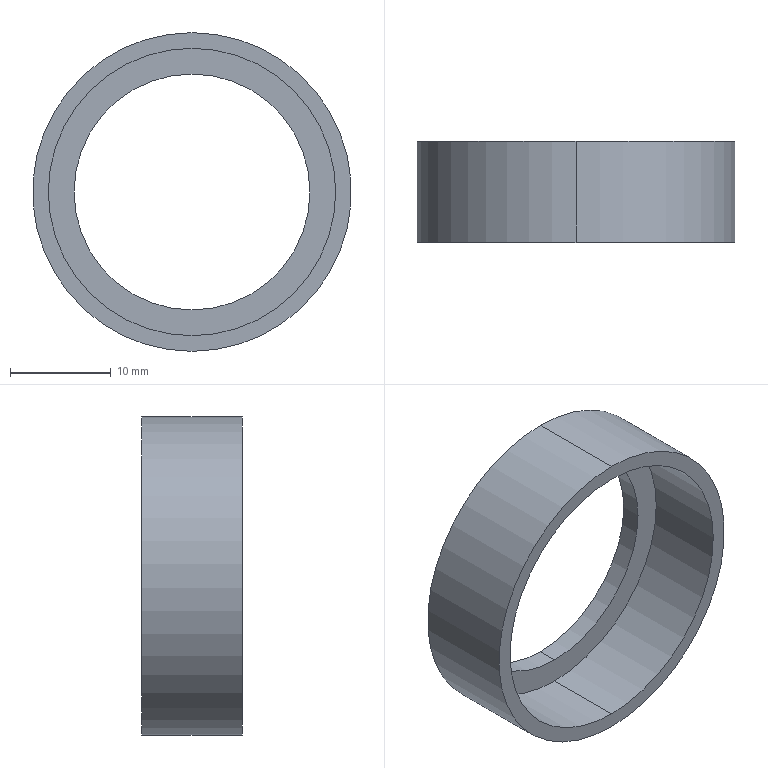Part | STEP file | P2858E27_RING_DICHT | 1 solid | 9 faces | box 31.6 x 10 x 31.6 mm | volume 1879 mm3 | cylinder 6 | plane 3 | commonest cylinder face diameters 23.4 x2 28.5 x2 31.6 x2
STEP:
#1=CARTESIAN_POINT('',(0.,0.,0.));
#2=DIRECTION('',(0.,0.,1.));
#3=DIRECTION('',(1.,0.,0.));
#4=AXIS2_PLACEMENT_3D('',#1,#2,#3);
#5=CARTESIAN_POINT('',(0.,28.,-15.8));
#6=VERTEX_POINT('',#5);
#7=CARTESIAN_POINT('',(0.,28.,15.8));
#8=VERTEX_POINT('',#7);
#9=CARTESIAN_POINT('',(0.,28.,0.));
#10=DIRECTION('',(0.,-1.,0.));
#11=DIRECTION('',(0.,0.,-1.));
#12=AXIS2_PLACEMENT_3D('',#9,#10,#11);
#13=CIRCLE('',#12,15.8);
#14=CARTESIAN_POINT('',(0.,23.,0.));
#15=DIRECTION('',(0.,-1.,0.));
#16=DIRECTION('',(0.,0.,-1.));
#17=AXIS2_PLACEMENT_3D('',#14,#15,#16);
#18=CYLINDRICAL_SURFACE('',#17,15.8);
#19=CARTESIAN_POINT('',(0.,-5.));
#20=DIRECTION('',(1.,0.));
#21=VECTOR('',#20,1.);
#22=LINE('',#19,#21);
#23=(GEOMETRIC_REPRESENTATION_CONTEXT(2)PARAMETRIC_REPRESENTATION_CONTEXT()REPRESENTATION_CONTEXT('',''));
#24=DEFINITIONAL_REPRESENTATION('',(#22),#23);
#25=PCURVE('',#18,#24);
#26=CARTESIAN_POINT('',(-13.75,28.,0.));
#27=DIRECTION('',(0.,-1.,0.));
#28=DIRECTION('',(0.,0.,-1.));
#29=AXIS2_PLACEMENT_3D('',#26,#27,#28);
#30=PLANE('',#29);
#31=CARTESIAN_POINT('',(0.,13.75));
#32=DIRECTION('',(1.,0.));
#33=AXIS2_PLACEMENT_2D('',#31,#32);
#34=CIRCLE('',#33,15.8);
#35=(GEOMETRIC_REPRESENTATION_CONTEXT(2)PARAMETRIC_REPRESENTATION_CONTEXT()REPRESENTATION_CONTEXT('',''));
#36=DEFINITIONAL_REPRESENTATION('',(#34),#35);
#37=PCURVE('',#30,#36);
#38=SURFACE_CURVE('',#13,(#25,#37),.PCURVE_S1.);
#39=EDGE_CURVE('',#6,#8,#38,.T.);
#40=ORIENTED_EDGE('',*,*,#39,.T.);
#41=CARTESIAN_POINT('',(0.,18.,15.8));
#42=VERTEX_POINT('',#41);
#43=CARTESIAN_POINT('',(0.,23.,15.8));
#44=DIRECTION('',(0.,-1.,0.));
#45=VECTOR('',#44,1.);
#46=LINE('',#43,#45);
#47=CARTESIAN_POINT('',(3.142,0.));
#48=DIRECTION('',(0.,1.));
#49=VECTOR('',#48,1.);
#50=LINE('',#47,#49);
#51=(GEOMETRIC_REPRESENTATION_CONTEXT(2)PARAMETRIC_REPRESENTATION_CONTEXT()REPRESENTATION_CONTEXT('',''));
#52=DEFINITIONAL_REPRESENTATION('',(#50),#51);
#53=PCURVE('',#18,#52);
#54=CARTESIAN_POINT('',(0.,23.,0.));
#55=DIRECTION('',(0.,-1.,0.));
#56=DIRECTION('',(0.,0.,-1.));
#57=AXIS2_PLACEMENT_3D('',#54,#55,#56);
#58=CYLINDRICAL_SURFACE('',#57,15.8);
#59=CARTESIAN_POINT('',(3.142,0.));
#60=DIRECTION('',(0.,1.));
#61=VECTOR('',#60,1.);
#62=LINE('',#59,#61);
#63=(GEOMETRIC_REPRESENTATION_CONTEXT(2)PARAMETRIC_REPRESENTATION_CONTEXT()REPRESENTATION_CONTEXT('',''));
#64=DEFINITIONAL_REPRESENTATION('',(#62),#63);
#65=PCURVE('',#58,#64);
#66=SURFACE_CURVE('',#46,(#53,#65),.PCURVE_S1.);
#67=EDGE_CURVE('',#8,#42,#66,.T.);
#68=ORIENTED_EDGE('',*,*,#67,.T.);
#69=CARTESIAN_POINT('',(0.,18.,-15.8));
#70=VERTEX_POINT('',#69);
#71=CARTESIAN_POINT('',(0.,18.,0.));
#72=DIRECTION('',(0.,1.,0.));
#73=DIRECTION('',(0.,0.,-1.));
#74=AXIS2_PLACEMENT_3D('',#71,#72,#73);
#75=CIRCLE('',#74,15.8);
#76=CARTESIAN_POINT('',(6.283,5.));
#77=DIRECTION('',(-1.,0.));
#78=VECTOR('',#77,1.);
#79=LINE('',#76,#78);
#80=(GEOMETRIC_REPRESENTATION_CONTEXT(2)PARAMETRIC_REPRESENTATION_CONTEXT()REPRESENTATION_CONTEXT('',''));
#81=DEFINITIONAL_REPRESENTATION('',(#79),#80);
#82=PCURVE('',#18,#81);
#83=CARTESIAN_POINT('',(-15.025,18.,0.));
#84=DIRECTION('',(0.,-1.,0.));
#85=DIRECTION('',(0.,0.,-1.));
#86=AXIS2_PLACEMENT_3D('',#83,#84,#85);
#87=PLANE('',#86);
#88=CARTESIAN_POINT('',(15.8,15.025));
#89=CARTESIAN_POINT('',(15.8,-12.341));
#90=CARTESIAN_POINT('',(-7.9,1.342));
#91=CARTESIAN_POINT('',(-31.6,15.025));
#92=CARTESIAN_POINT('',(-7.9,28.708));
#93=CARTESIAN_POINT('',(15.8,42.391));
#94=CARTESIAN_POINT('',(15.8,15.025));
#95=(BOUNDED_CURVE()B_SPLINE_CURVE(2,(#88,#89,#90,#91,#92,#93,#94),.UNSPECIFIED.,.T.,.F.)B_SPLINE_CURVE_WITH_KNOTS((1,2,2,2,2,1),(-2.094,0.,2.094,4.189,6.283,8.378),.UNSPECIFIED.)CURVE()GEOMETRIC_REPRESENTATION_ITEM()RATIONAL_B_SPLINE_CURVE((1.,0.5,1.,0.5,1.,0.5,1.))REPRESENTATION_ITEM(''));
#96=(GEOMETRIC_REPRESENTATION_CONTEXT(2)PARAMETRIC_REPRESENTATION_CONTEXT()REPRESENTATION_CONTEXT('',''));
#97=DEFINITIONAL_REPRESENTATION('',(#95),#96);
#98=PCURVE('',#87,#97);
#99=SURFACE_CURVE('',#75,(#82,#98),.PCURVE_S1.);
#100=EDGE_CURVE('',#42,#70,#99,.T.);
#101=ORIENTED_EDGE('',*,*,#100,.T.);
#102=CARTESIAN_POINT('',(0.,23.,-15.8));
#103=DIRECTION('',(0.,-1.,0.));
#104=VECTOR('',#103,1.);
#105=LINE('',#102,#104);
#106=CARTESIAN_POINT('',(0.,0.));
#107=DIRECTION('',(0.,1.));
#108=VECTOR('',#107,1.);
#109=LINE('',#106,#108);
#110=(GEOMETRIC_REPRESENTATION_CONTEXT(2)PARAMETRIC_REPRESENTATION_CONTEXT()REPRESENTATION_CONTEXT('',''));
#111=DEFINITIONAL_REPRESENTATION('',(#109),#110);
#112=PCURVE('',#18,#111);
#113=CARTESIAN_POINT('',(6.283,0.));
#114=DIRECTION('',(0.,1.));
#115=VECTOR('',#114,1.);
#116=LINE('',#113,#115);
#117=(GEOMETRIC_REPRESENTATION_CONTEXT(2)PARAMETRIC_REPRESENTATION_CONTEXT()REPRESENTATION_CONTEXT('',''));
#118=DEFINITIONAL_REPRESENTATION('',(#116),#117);
#119=PCURVE('',#58,#118);
#120=SURFACE_CURVE('',#105,(#112,#119),.PCURVE_S1.);
#121=EDGE_CURVE('',#6,#70,#120,.T.);
#122=ORIENTED_EDGE('',*,*,#121,.F.);
#123=EDGE_LOOP('',(#40,#68,#101,#122));
#124=FACE_BOUND('',#123,.T.);
#125=ADVANCED_FACE('',(#124),#18,.T.);
#126=CARTESIAN_POINT('',(0.,28.,-11.7));
#127=VERTEX_POINT('',#126);
#128=CARTESIAN_POINT('',(0.,26.,-11.7));
#129=VERTEX_POINT('',#128);
#130=CARTESIAN_POINT('',(0.,27.,-11.7));
#131=DIRECTION('',(0.,-1.,0.));
#132=VECTOR('',#131,1.);
#133=LINE('',#130,#132);
#134=CARTESIAN_POINT('',(0.,27.,0.));
#135=DIRECTION('',(0.,-1.,0.));
#136=DIRECTION('',(0.,0.,-1.));
#137=AXIS2_PLACEMENT_3D('',#134,#135,#136);
#138=CYLINDRICAL_SURFACE('',#137,11.7);
#139=CARTESIAN_POINT('',(6.283,0.));
#140=DIRECTION('',(0.,1.));
#141=VECTOR('',#140,1.);
#142=LINE('',#139,#141);
#143=(GEOMETRIC_REPRESENTATION_CONTEXT(2)PARAMETRIC_REPRESENTATION_CONTEXT()REPRESENTATION_CONTEXT('',''));
#144=DEFINITIONAL_REPRESENTATION('',(#142),#143);
#145=PCURVE('',#138,#144);
#146=CARTESIAN_POINT('',(0.,27.,0.));
#147=DIRECTION('',(0.,-1.,0.));
#148=DIRECTION('',(0.,0.,-1.));
#149=AXIS2_PLACEMENT_3D('',#146,#147,#148);
#150=CYLINDRICAL_SURFACE('',#149,11.7);
#151=CARTESIAN_POINT('',(0.,0.));
#152=DIRECTION('',(0.,1.));
#153=VECTOR('',#152,1.);
#154=LINE('',#151,#153);
#155=(GEOMETRIC_REPRESENTATION_CONTEXT(2)PARAMETRIC_REPRESENTATION_CONTEXT()REPRESENTATION_CONTEXT('',''));
#156=DEFINITIONAL_REPRESENTATION('',(#154),#155);
#157=PCURVE('',#150,#156);
#158=SURFACE_CURVE('',#133,(#145,#157),.PCURVE_S1.);
#159=EDGE_CURVE('',#127,#129,#158,.T.);
#160=ORIENTED_EDGE('',*,*,#159,.T.);
#161=CARTESIAN_POINT('',(0.,26.,11.7));
#162=VERTEX_POINT('',#161);
#163=CARTESIAN_POINT('',(0.,26.,0.));
#164=DIRECTION('',(0.,1.,0.));
#165=DIRECTION('',(0.,0.,-1.));
#166=AXIS2_PLACEMENT_3D('',#163,#164,#165);
#167=CIRCLE('',#166,11.7);
#168=CARTESIAN_POINT('',(6.283,1.));
#169=DIRECTION('',(-1.,0.));
#170=VECTOR('',#169,1.);
#171=LINE('',#168,#170);
#172=(GEOMETRIC_REPRESENTATION_CONTEXT(2)PARAMETRIC_REPRESENTATION_CONTEXT()REPRESENTATION_CONTEXT('',''));
#173=DEFINITIONAL_REPRESENTATION('',(#171),#172);
#174=PCURVE('',#138,#173);
#175=CARTESIAN_POINT('',(-12.975,26.,0.));
#176=DIRECTION('',(0.,-1.,0.));
#177=DIRECTION('',(0.,0.,-1.));
#178=AXIS2_PLACEMENT_3D('',#175,#176,#177);
#179=PLANE('',#178);
#180=CARTESIAN_POINT('',(11.7,12.975));
#181=CARTESIAN_POINT('',(11.7,-7.29));
#182=CARTESIAN_POINT('',(-5.85,2.843));
#183=CARTESIAN_POINT('',(-23.4,12.975));
#184=CARTESIAN_POINT('',(-5.85,23.107));
#185=CARTESIAN_POINT('',(11.7,33.24));
#186=CARTESIAN_POINT('',(11.7,12.975));
#187=(BOUNDED_CURVE()B_SPLINE_CURVE(2,(#180,#181,#182,#183,#184,#185,#186),.UNSPECIFIED.,.T.,.F.)B_SPLINE_CURVE_WITH_KNOTS((1,2,2,2,2,1),(-2.094,0.,2.094,4.189,6.283,8.378),.UNSPECIFIED.)CURVE()GEOMETRIC_REPRESENTATION_ITEM()RATIONAL_B_SPLINE_CURVE((1.,0.5,1.,0.5,1.,0.5,1.))REPRESENTATION_ITEM(''));
#188=(GEOMETRIC_REPRESENTATION_CONTEXT(2)PARAMETRIC_REPRESENTATION_CONTEXT()REPRESENTATION_CONTEXT('',''));
#189=DEFINITIONAL_REPRESENTATION('',(#187),#188);
#190=PCURVE('',#179,#189);
#191=SURFACE_CURVE('',#167,(#174,#190),.PCURVE_S1.);
#192=EDGE_CURVE('',#129,#162,#191,.T.);
#193=ORIENTED_EDGE('',*,*,#192,.T.);
#194=CARTESIAN_POINT('',(0.,28.,11.7));
#195=VERTEX_POINT('',#194);
#196=CARTESIAN_POINT('',(0.,27.,11.7));
#197=DIRECTION('',(0.,-1.,0.));
#198=VECTOR('',#197,1.);
#199=LINE('',#196,#198);
#200=CARTESIAN_POINT('',(3.142,0.));
#201=DIRECTION('',(0.,1.));
#202=VECTOR('',#201,1.);
#203=LINE('',#200,#202);
#204=(GEOMETRIC_REPRESENTATION_CONTEXT(2)PARAMETRIC_REPRESENTATION_CONTEXT()REPRESENTATION_CONTEXT('',''));
#205=DEFINITIONAL_REPRESENTATION('',(#203),#204);
#206=PCURVE('',#138,#205);
#207=CARTESIAN_POINT('',(3.142,0.));
#208=DIRECTION('',(0.,1.));
#209=VECTOR('',#208,1.);
#210=LINE('',#207,#209);
#211=(GEOMETRIC_REPRESENTATION_CONTEXT(2)PARAMETRIC_REPRESENTATION_CONTEXT()REPRESENTATION_CONTEXT('',''));
#212=DEFINITIONAL_REPRESENTATION('',(#210),#211);
#213=PCURVE('',#150,#212);
#214=SURFACE_CURVE('',#199,(#206,#213),.PCURVE_S1.);
#215=EDGE_CURVE('',#195,#162,#214,.T.);
#216=ORIENTED_EDGE('',*,*,#215,.F.);
#217=CARTESIAN_POINT('',(0.,28.,0.));
#218=DIRECTION('',(0.,1.,0.));
#219=DIRECTION('',(0.,0.,-1.));
#220=AXIS2_PLACEMENT_3D('',#217,#218,#219);
#221=CIRCLE('',#220,11.7);
#222=CARTESIAN_POINT('',(6.283,-1.));
#223=DIRECTION('',(-1.,0.));
#224=VECTOR('',#223,1.);
#225=LINE('',#222,#224);
#226=(GEOMETRIC_REPRESENTATION_CONTEXT(2)PARAMETRIC_REPRESENTATION_CONTEXT()REPRESENTATION_CONTEXT('',''));
#227=DEFINITIONAL_REPRESENTATION('',(#225),#226);
#228=PCURVE('',#138,#227);
#229=CARTESIAN_POINT('',(11.7,13.75));
#230=CARTESIAN_POINT('',(11.7,-6.515));
#231=CARTESIAN_POINT('',(-5.85,3.618));
#232=CARTESIAN_POINT('',(-23.4,13.75));
#233=CARTESIAN_POINT('',(-5.85,23.882));
#234=CARTESIAN_POINT('',(11.7,34.015));
#235=CARTESIAN_POINT('',(11.7,13.75));
#236=(BOUNDED_CURVE()B_SPLINE_CURVE(2,(#229,#230,#231,#232,#233,#234,#235),.UNSPECIFIED.,.T.,.F.)B_SPLINE_CURVE_WITH_KNOTS((1,2,2,2,2,1),(-2.094,0.,2.094,4.189,6.283,8.378),.UNSPECIFIED.)CURVE()GEOMETRIC_REPRESENTATION_ITEM()RATIONAL_B_SPLINE_CURVE((1.,0.5,1.,0.5,1.,0.5,1.))REPRESENTATION_ITEM(''));
#237=(GEOMETRIC_REPRESENTATION_CONTEXT(2)PARAMETRIC_REPRESENTATION_CONTEXT()REPRESENTATION_CONTEXT('',''));
#238=DEFINITIONAL_REPRESENTATION('',(#236),#237);
#239=PCURVE('',#30,#238);
#240=SURFACE_CURVE('',#221,(#228,#239),.PCURVE_S1.);
#241=EDGE_CURVE('',#127,#195,#240,.T.);
#242=ORIENTED_EDGE('',*,*,#241,.F.);
#243=EDGE_LOOP('',(#160,#193,#216,#242));
#244=FACE_BOUND('',#243,.F.);
#245=ADVANCED_FACE('',(#244),#138,.F.);
#246=CARTESIAN_POINT('',(0.,26.,-14.25));
#247=VERTEX_POINT('',#246);
#248=CARTESIAN_POINT('',(0.,18.,-14.25));
#249=VERTEX_POINT('',#248);
#250=CARTESIAN_POINT('',(0.,22.,-14.25));
#251=DIRECTION('',(0.,-1.,0.));
#252=VECTOR('',#251,1.);
#253=LINE('',#250,#252);
#254=CARTESIAN_POINT('',(0.,22.,0.));
#255=DIRECTION('',(0.,-1.,0.));
#256=DIRECTION('',(0.,0.,-1.));
#257=AXIS2_PLACEMENT_3D('',#254,#255,#256);
#258=CYLINDRICAL_SURFACE('',#257,14.25);
#259=CARTESIAN_POINT('',(6.283,0.));
#260=DIRECTION('',(0.,1.));
#261=VECTOR('',#260,1.);
#262=LINE('',#259,#261);
#263=(GEOMETRIC_REPRESENTATION_CONTEXT(2)PARAMETRIC_REPRESENTATION_CONTEXT()REPRESENTATION_CONTEXT('',''));
#264=DEFINITIONAL_REPRESENTATION('',(#262),#263);
#265=PCURVE('',#258,#264);
#266=CARTESIAN_POINT('',(0.,22.,0.));
#267=DIRECTION('',(0.,-1.,0.));
#268=DIRECTION('',(0.,0.,-1.));
#269=AXIS2_PLACEMENT_3D('',#266,#267,#268);
#270=CYLINDRICAL_SURFACE('',#269,14.25);
#271=CARTESIAN_POINT('',(0.,0.));
#272=DIRECTION('',(0.,1.));
#273=VECTOR('',#272,1.);
#274=LINE('',#271,#273);
#275=(GEOMETRIC_REPRESENTATION_CONTEXT(2)PARAMETRIC_REPRESENTATION_CONTEXT()REPRESENTATION_CONTEXT('',''));
#276=DEFINITIONAL_REPRESENTATION('',(#274),#275);
#277=PCURVE('',#270,#276);
#278=SURFACE_CURVE('',#253,(#265,#277),.PCURVE_S1.);
#279=EDGE_CURVE('',#247,#249,#278,.T.);
#280=ORIENTED_EDGE('',*,*,#279,.T.);
#281=CARTESIAN_POINT('',(0.,18.,14.25));
#282=VERTEX_POINT('',#281);
#283=CARTESIAN_POINT('',(0.,18.,0.));
#284=DIRECTION('',(0.,1.,0.));
#285=DIRECTION('',(0.,0.,-1.));
#286=AXIS2_PLACEMENT_3D('',#283,#284,#285);
#287=CIRCLE('',#286,14.25);
#288=CARTESIAN_POINT('',(6.283,4.));
#289=DIRECTION('',(-1.,0.));
#290=VECTOR('',#289,1.);
#291=LINE('',#288,#290);
#292=(GEOMETRIC_REPRESENTATION_CONTEXT(2)PARAMETRIC_REPRESENTATION_CONTEXT()REPRESENTATION_CONTEXT('',''));
#293=DEFINITIONAL_REPRESENTATION('',(#291),#292);
#294=PCURVE('',#258,#293);
#295=CARTESIAN_POINT('',(14.25,15.025));
#296=CARTESIAN_POINT('',(14.25,-9.657));
#297=CARTESIAN_POINT('',(-7.125,2.684));
#298=CARTESIAN_POINT('',(-28.5,15.025));
#299=CARTESIAN_POINT('',(-7.125,27.366));
#300=CARTESIAN_POINT('',(14.25,39.707));
#301=CARTESIAN_POINT('',(14.25,15.025));
#302=(BOUNDED_CURVE()B_SPLINE_CURVE(2,(#295,#296,#297,#298,#299,#300,#301),.UNSPECIFIED.,.T.,.F.)B_SPLINE_CURVE_WITH_KNOTS((1,2,2,2,2,1),(-2.094,0.,2.094,4.189,6.283,8.378),.UNSPECIFIED.)CURVE()GEOMETRIC_REPRESENTATION_ITEM()RATIONAL_B_SPLINE_CURVE((1.,0.5,1.,0.5,1.,0.5,1.))REPRESENTATION_ITEM(''));
#303=(GEOMETRIC_REPRESENTATION_CONTEXT(2)PARAMETRIC_REPRESENTATION_CONTEXT()REPRESENTATION_CONTEXT('',''));
#304=DEFINITIONAL_REPRESENTATION('',(#302),#303);
#305=PCURVE('',#87,#304);
#306=SURFACE_CURVE('',#287,(#294,#305),.PCURVE_S1.);
#307=EDGE_CURVE('',#249,#282,#306,.T.);
#308=ORIENTED_EDGE('',*,*,#307,.T.);
#309=CARTESIAN_POINT('',(0.,26.,14.25));
#310=VERTEX_POINT('',#309);
#311=CARTESIAN_POINT('',(0.,22.,14.25));
#312=DIRECTION('',(0.,-1.,0.));
#313=VECTOR('',#312,1.);
#314=LINE('',#311,#313);
#315=CARTESIAN_POINT('',(3.142,0.));
#316=DIRECTION('',(0.,1.));
#317=VECTOR('',#316,1.);
#318=LINE('',#315,#317);
#319=(GEOMETRIC_REPRESENTATION_CONTEXT(2)PARAMETRIC_REPRESENTATION_CONTEXT()REPRESENTATION_CONTEXT('',''));
#320=DEFINITIONAL_REPRESENTATION('',(#318),#319);
#321=PCURVE('',#258,#320);
#322=CARTESIAN_POINT('',(3.142,0.));
#323=DIRECTION('',(0.,1.));
#324=VECTOR('',#323,1.);
#325=LINE('',#322,#324);
#326=(GEOMETRIC_REPRESENTATION_CONTEXT(2)PARAMETRIC_REPRESENTATION_CONTEXT()REPRESENTATION_CONTEXT('',''));
#327=DEFINITIONAL_REPRESENTATION('',(#325),#326);
#328=PCURVE('',#270,#327);
#329=SURFACE_CURVE('',#314,(#321,#328),.PCURVE_S1.);
#330=EDGE_CURVE('',#310,#282,#329,.T.);
#331=ORIENTED_EDGE('',*,*,#330,.F.);
#332=CARTESIAN_POINT('',(0.,26.,0.));
#333=DIRECTION('',(0.,-1.,0.));
#334=DIRECTION('',(0.,0.,-1.));
#335=AXIS2_PLACEMENT_3D('',#332,#333,#334);
#336=CIRCLE('',#335,14.25);
#337=CARTESIAN_POINT('',(0.,-4.));
#338=DIRECTION('',(1.,0.));
#339=VECTOR('',#338,1.);
#340=LINE('',#337,#339);
#341=(GEOMETRIC_REPRESENTATION_CONTEXT(2)PARAMETRIC_REPRESENTATION_CONTEXT()REPRESENTATION_CONTEXT('',''));
#342=DEFINITIONAL_REPRESENTATION('',(#340),#341);
#343=PCURVE('',#258,#342);
#344=CARTESIAN_POINT('',(0.,12.975));
#345=DIRECTION('',(1.,0.));
#346=AXIS2_PLACEMENT_2D('',#344,#345);
#347=CIRCLE('',#346,14.25);
#348=(GEOMETRIC_REPRESENTATION_CONTEXT(2)PARAMETRIC_REPRESENTATION_CONTEXT()REPRESENTATION_CONTEXT('',''));
#349=DEFINITIONAL_REPRESENTATION('',(#347),#348);
#350=PCURVE('',#179,#349);
#351=SURFACE_CURVE('',#336,(#343,#350),.PCURVE_S1.);
#352=EDGE_CURVE('',#310,#247,#351,.T.);
#353=ORIENTED_EDGE('',*,*,#352,.T.);
#354=EDGE_LOOP('',(#280,#308,#331,#353));
#355=FACE_BOUND('',#354,.F.);
#356=ADVANCED_FACE('',(#355),#258,.F.);
#357=ORIENTED_EDGE('',*,*,#192,.T.);
#358=CARTESIAN_POINT('',(0.,26.,0.));
#359=DIRECTION('',(0.,1.,0.));
#360=DIRECTION('',(0.,0.,-1.));
#361=AXIS2_PLACEMENT_3D('',#358,#359,#360);
#362=CIRCLE('',#361,11.7);
#363=CARTESIAN_POINT('',(11.7,12.975));
#364=CARTESIAN_POINT('',(11.7,-7.29));
#365=CARTESIAN_POINT('',(-5.85,2.843));
#366=CARTESIAN_POINT('',(-23.4,12.975));
#367=CARTESIAN_POINT('',(-5.85,23.107));
#368=CARTESIAN_POINT('',(11.7,33.24));
#369=CARTESIAN_POINT('',(11.7,12.975));
#370=(BOUNDED_CURVE()B_SPLINE_CURVE(2,(#363,#364,#365,#366,#367,#368,#369),.UNSPECIFIED.,.T.,.F.)B_SPLINE_CURVE_WITH_KNOTS((1,2,2,2,2,1),(-2.094,0.,2.094,4.189,6.283,8.378),.UNSPECIFIED.)CURVE()GEOMETRIC_REPRESENTATION_ITEM()RATIONAL_B_SPLINE_CURVE((1.,0.5,1.,0.5,1.,0.5,1.))REPRESENTATION_ITEM(''));
#371=(GEOMETRIC_REPRESENTATION_CONTEXT(2)PARAMETRIC_REPRESENTATION_CONTEXT()REPRESENTATION_CONTEXT('',''));
#372=DEFINITIONAL_REPRESENTATION('',(#370),#371);
#373=PCURVE('',#179,#372);
#374=CARTESIAN_POINT('',(6.283,1.));
#375=DIRECTION('',(-1.,0.));
#376=VECTOR('',#375,1.);
#377=LINE('',#374,#376);
#378=(GEOMETRIC_REPRESENTATION_CONTEXT(2)PARAMETRIC_REPRESENTATION_CONTEXT()REPRESENTATION_CONTEXT('',''));
#379=DEFINITIONAL_REPRESENTATION('',(#377),#378);
#380=PCURVE('',#150,#379);
#381=SURFACE_CURVE('',#362,(#373,#380),.PCURVE_S1.);
#382=EDGE_CURVE('',#162,#129,#381,.T.);
#383=ORIENTED_EDGE('',*,*,#382,.T.);
#384=EDGE_LOOP('',(#357,#383));
#385=FACE_BOUND('',#384,.T.);
#386=CARTESIAN_POINT('',(0.,26.,0.));
#387=DIRECTION('',(0.,-1.,0.));
#388=DIRECTION('',(0.,0.,-1.));
#389=AXIS2_PLACEMENT_3D('',#386,#387,#388);
#390=CIRCLE('',#389,14.25);
#391=CARTESIAN_POINT('',(0.,12.975));
#392=DIRECTION('',(1.,0.));
#393=AXIS2_PLACEMENT_2D('',#391,#392);
#394=CIRCLE('',#393,14.25);
#395=(GEOMETRIC_REPRESENTATION_CONTEXT(2)PARAMETRIC_REPRESENTATION_CONTEXT()REPRESENTATION_CONTEXT('',''));
#396=DEFINITIONAL_REPRESENTATION('',(#394),#395);
#397=PCURVE('',#179,#396);
#398=CARTESIAN_POINT('',(0.,-4.));
#399=DIRECTION('',(1.,0.));
#400=VECTOR('',#399,1.);
#401=LINE('',#398,#400);
#402=(GEOMETRIC_REPRESENTATION_CONTEXT(2)PARAMETRIC_REPRESENTATION_CONTEXT()REPRESENTATION_CONTEXT('',''));
#403=DEFINITIONAL_REPRESENTATION('',(#401),#402);
#404=PCURVE('',#270,#403);
#405=SURFACE_CURVE('',#390,(#397,#404),.PCURVE_S1.);
#406=EDGE_CURVE('',#247,#310,#405,.T.);
#407=ORIENTED_EDGE('',*,*,#406,.T.);
#408=ORIENTED_EDGE('',*,*,#352,.T.);
#409=EDGE_LOOP('',(#407,#408));
#410=FACE_BOUND('',#409,.T.);
#411=ADVANCED_FACE('',(#385,#410),#179,.T.);
#412=CARTESIAN_POINT('',(0.,18.,0.));
#413=DIRECTION('',(0.,1.,0.));
#414=DIRECTION('',(0.,0.,-1.));
#415=AXIS2_PLACEMENT_3D('',#412,#413,#414);
#416=CIRCLE('',#415,14.25);
#417=CARTESIAN_POINT('',(6.283,4.));
#418=DIRECTION('',(-1.,0.));
#419=VECTOR('',#418,1.);
#420=LINE('',#417,#419);
#421=(GEOMETRIC_REPRESENTATION_CONTEXT(2)PARAMETRIC_REPRESENTATION_CONTEXT()REPRESENTATION_CONTEXT('',''));
#422=DEFINITIONAL_REPRESENTATION('',(#420),#421);
#423=PCURVE('',#270,#422);
#424=CARTESIAN_POINT('',(14.25,15.025));
#425=CARTESIAN_POINT('',(14.25,-9.657));
#426=CARTESIAN_POINT('',(-7.125,2.684));
#427=CARTESIAN_POINT('',(-28.5,15.025));
#428=CARTESIAN_POINT('',(-7.125,27.366));
#429=CARTESIAN_POINT('',(14.25,39.707));
#430=CARTESIAN_POINT('',(14.25,15.025));
#431=(BOUNDED_CURVE()B_SPLINE_CURVE(2,(#424,#425,#426,#427,#428,#429,#430),.UNSPECIFIED.,.T.,.F.)B_SPLINE_CURVE_WITH_KNOTS((1,2,2,2,2,1),(-2.094,0.,2.094,4.189,6.283,8.378),.UNSPECIFIED.)CURVE()GEOMETRIC_REPRESENTATION_ITEM()RATIONAL_B_SPLINE_CURVE((1.,0.5,1.,0.5,1.,0.5,1.))REPRESENTATION_ITEM(''));
#432=(GEOMETRIC_REPRESENTATION_CONTEXT(2)PARAMETRIC_REPRESENTATION_CONTEXT()REPRESENTATION_CONTEXT('',''));
#433=DEFINITIONAL_REPRESENTATION('',(#431),#432);
#434=PCURVE('',#87,#433);
#435=SURFACE_CURVE('',#416,(#423,#434),.PCURVE_S1.);
#436=EDGE_CURVE('',#282,#249,#435,.T.);
#437=ORIENTED_EDGE('',*,*,#436,.T.);
#438=ORIENTED_EDGE('',*,*,#279,.F.);
#439=ORIENTED_EDGE('',*,*,#406,.T.);
#440=ORIENTED_EDGE('',*,*,#330,.T.);
#441=EDGE_LOOP('',(#437,#438,#439,#440));
#442=FACE_BOUND('',#441,.F.);
#443=ADVANCED_FACE('',(#442),#270,.F.);
#444=ORIENTED_EDGE('',*,*,#382,.T.);
#445=ORIENTED_EDGE('',*,*,#159,.F.);
#446=CARTESIAN_POINT('',(0.,28.,0.));
#447=DIRECTION('',(0.,1.,0.));
#448=DIRECTION('',(0.,0.,-1.));
#449=AXIS2_PLACEMENT_3D('',#446,#447,#448);
#450=CIRCLE('',#449,11.7);
#451=CARTESIAN_POINT('',(6.283,-1.));
#452=DIRECTION('',(-1.,0.));
#453=VECTOR('',#452,1.);
#454=LINE('',#451,#453);
#455=(GEOMETRIC_REPRESENTATION_CONTEXT(2)PARAMETRIC_REPRESENTATION_CONTEXT()REPRESENTATION_CONTEXT('',''));
#456=DEFINITIONAL_REPRESENTATION('',(#454),#455);
#457=PCURVE('',#150,#456);
#458=CARTESIAN_POINT('',(11.7,13.75));
#459=CARTESIAN_POINT('',(11.7,-6.515));
#460=CARTESIAN_POINT('',(-5.85,3.618));
#461=CARTESIAN_POINT('',(-23.4,13.75));
#462=CARTESIAN_POINT('',(-5.85,23.882));
#463=CARTESIAN_POINT('',(11.7,34.015));
#464=CARTESIAN_POINT('',(11.7,13.75));
#465=(BOUNDED_CURVE()B_SPLINE_CURVE(2,(#458,#459,#460,#461,#462,#463,#464),.UNSPECIFIED.,.T.,.F.)B_SPLINE_CURVE_WITH_KNOTS((1,2,2,2,2,1),(-2.094,0.,2.094,4.189,6.283,8.378),.UNSPECIFIED.)CURVE()GEOMETRIC_REPRESENTATION_ITEM()RATIONAL_B_SPLINE_CURVE((1.,0.5,1.,0.5,1.,0.5,1.))REPRESENTATION_ITEM(''));
#466=(GEOMETRIC_REPRESENTATION_CONTEXT(2)PARAMETRIC_REPRESENTATION_CONTEXT()REPRESENTATION_CONTEXT('',''));
#467=DEFINITIONAL_REPRESENTATION('',(#465),#466);
#468=PCURVE('',#30,#467);
#469=SURFACE_CURVE('',#450,(#457,#468),.PCURVE_S1.);
#470=EDGE_CURVE('',#195,#127,#469,.T.);
#471=ORIENTED_EDGE('',*,*,#470,.F.);
#472=ORIENTED_EDGE('',*,*,#215,.T.);
#473=EDGE_LOOP('',(#444,#445,#471,#472));
#474=FACE_BOUND('',#473,.F.);
#475=ADVANCED_FACE('',(#474),#150,.F.);
#476=ORIENTED_EDGE('',*,*,#307,.T.);
#477=ORIENTED_EDGE('',*,*,#436,.T.);
#478=EDGE_LOOP('',(#476,#477));
#479=FACE_BOUND('',#478,.T.);
#480=CARTESIAN_POINT('',(0.,18.,0.));
#481=DIRECTION('',(0.,1.,0.));
#482=DIRECTION('',(0.,0.,-1.));
#483=AXIS2_PLACEMENT_3D('',#480,#481,#482);
#484=CIRCLE('',#483,15.8);
#485=CARTESIAN_POINT('',(15.8,15.025));
#486=CARTESIAN_POINT('',(15.8,-12.341));
#487=CARTESIAN_POINT('',(-7.9,1.342));
#488=CARTESIAN_POINT('',(-31.6,15.025));
#489=CARTESIAN_POINT('',(-7.9,28.708));
#490=CARTESIAN_POINT('',(15.8,42.391));
#491=CARTESIAN_POINT('',(15.8,15.025));
#492=(BOUNDED_CURVE()B_SPLINE_CURVE(2,(#485,#486,#487,#488,#489,#490,#491),.UNSPECIFIED.,.T.,.F.)B_SPLINE_CURVE_WITH_KNOTS((1,2,2,2,2,1),(-2.094,0.,2.094,4.189,6.283,8.378),.UNSPECIFIED.)CURVE()GEOMETRIC_REPRESENTATION_ITEM()RATIONAL_B_SPLINE_CURVE((1.,0.5,1.,0.5,1.,0.5,1.))REPRESENTATION_ITEM(''));
#493=(GEOMETRIC_REPRESENTATION_CONTEXT(2)PARAMETRIC_REPRESENTATION_CONTEXT()REPRESENTATION_CONTEXT('',''));
#494=DEFINITIONAL_REPRESENTATION('',(#492),#493);
#495=PCURVE('',#87,#494);
#496=CARTESIAN_POINT('',(6.283,5.));
#497=DIRECTION('',(-1.,0.));
#498=VECTOR('',#497,1.);
#499=LINE('',#496,#498);
#500=(GEOMETRIC_REPRESENTATION_CONTEXT(2)PARAMETRIC_REPRESENTATION_CONTEXT()REPRESENTATION_CONTEXT('',''));
#501=DEFINITIONAL_REPRESENTATION('',(#499),#500);
#502=PCURVE('',#58,#501);
#503=SURFACE_CURVE('',#484,(#495,#502),.PCURVE_S1.);
#504=EDGE_CURVE('',#70,#42,#503,.T.);
#505=ORIENTED_EDGE('',*,*,#504,.F.);
#506=ORIENTED_EDGE('',*,*,#100,.F.);
#507=EDGE_LOOP('',(#505,#506));
#508=FACE_BOUND('',#507,.T.);
#509=ADVANCED_FACE('',(#479,#508),#87,.T.);
#510=ORIENTED_EDGE('',*,*,#241,.F.);
#511=ORIENTED_EDGE('',*,*,#470,.F.);
#512=EDGE_LOOP('',(#510,#511));
#513=FACE_BOUND('',#512,.T.);
#514=ORIENTED_EDGE('',*,*,#39,.F.);
#515=CARTESIAN_POINT('',(0.,28.,0.));
#516=DIRECTION('',(0.,-1.,0.));
#517=DIRECTION('',(0.,0.,-1.));
#518=AXIS2_PLACEMENT_3D('',#515,#516,#517);
#519=CIRCLE('',#518,15.8);
#520=CARTESIAN_POINT('',(0.,13.75));
#521=DIRECTION('',(1.,0.));
#522=AXIS2_PLACEMENT_2D('',#520,#521);
#523=CIRCLE('',#522,15.8);
#524=(GEOMETRIC_REPRESENTATION_CONTEXT(2)PARAMETRIC_REPRESENTATION_CONTEXT()REPRESENTATION_CONTEXT('',''));
#525=DEFINITIONAL_REPRESENTATION('',(#523),#524);
#526=PCURVE('',#30,#525);
#527=CARTESIAN_POINT('',(0.,-5.));
#528=DIRECTION('',(1.,0.));
#529=VECTOR('',#528,1.);
#530=LINE('',#527,#529);
#531=(GEOMETRIC_REPRESENTATION_CONTEXT(2)PARAMETRIC_REPRESENTATION_CONTEXT()REPRESENTATION_CONTEXT('',''));
#532=DEFINITIONAL_REPRESENTATION('',(#530),#531);
#533=PCURVE('',#58,#532);
#534=SURFACE_CURVE('',#519,(#526,#533),.PCURVE_S1.);
#535=EDGE_CURVE('',#8,#6,#534,.T.);
#536=ORIENTED_EDGE('',*,*,#535,.F.);
#537=EDGE_LOOP('',(#514,#536));
#538=FACE_BOUND('',#537,.T.);
#539=ADVANCED_FACE('',(#513,#538),#30,.F.);
#540=ORIENTED_EDGE('',*,*,#67,.F.);
#541=ORIENTED_EDGE('',*,*,#535,.T.);
#542=ORIENTED_EDGE('',*,*,#121,.T.);
#543=ORIENTED_EDGE('',*,*,#504,.T.);
#544=EDGE_LOOP('',(#540,#541,#542,#543));
#545=FACE_BOUND('',#544,.T.);
#546=ADVANCED_FACE('',(#545),#58,.T.);
#547=CLOSED_SHELL('',(#125,#245,#356,#411,#443,#475,#509,#539,#546));
#548=MANIFOLD_SOLID_BREP('',#547);
#549=(LENGTH_UNIT()NAMED_UNIT(*)SI_UNIT(.MILLI.,.METRE.));
#550=UNCERTAINTY_MEASURE_WITH_UNIT(LENGTH_MEASURE(0.0000001),#549,'','');
#551=(NAMED_UNIT(*)PLANE_ANGLE_UNIT()SI_UNIT($,.RADIAN.));
#552=(NAMED_UNIT(*)SI_UNIT($,.STERADIAN.)SOLID_ANGLE_UNIT());
#553=(GEOMETRIC_REPRESENTATION_CONTEXT(3)GLOBAL_UNCERTAINTY_ASSIGNED_CONTEXT((#550))GLOBAL_UNIT_ASSIGNED_CONTEXT((#549,#551,#552))REPRESENTATION_CONTEXT('',''));
#554=ADVANCED_BREP_SHAPE_REPRESENTATION('',(#4,#548),#553);